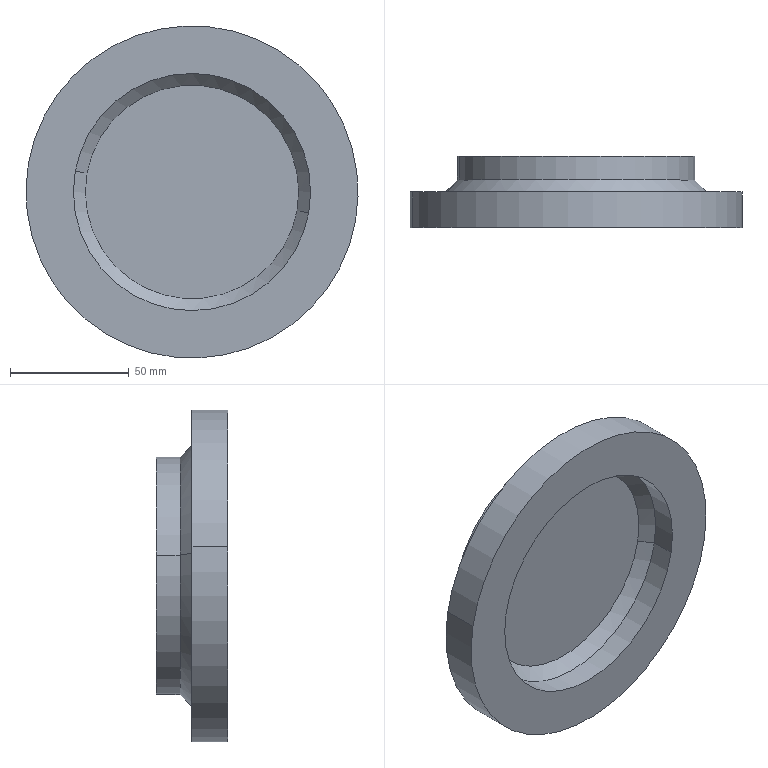Part | SolidWorks | features BaseBody 1 | 1 solid | 17 faces | box 140 x 30 x 140 mm | volume 231551 mm3 | cone 6 | cylinder 6 | plane 5 | commonest cylinder face diameters 100 x4 140 x2
STEP:
#1=CARTESIAN_POINT('',(224.832,513.635,261.862));
#2=VERTEX_POINT('',#1);
#3=CARTESIAN_POINT('',(214.987,523.635,263.616));
#4=VERTEX_POINT('',#3);
#5=CARTESIAN_POINT('',(224.832,513.635,261.862));
#6=DIRECTION('',(-0.6961,0.7071,0.1241));
#7=VECTOR('',#6,1000.);
#8=LINE('',#5,#7);
#9=EDGE_CURVE('',#2,#4,#8,.T.);
#10=ORIENTED_EDGE('',*,*,#9,.F.);
#11=CARTESIAN_POINT('',(244.522,513.635,258.352));
#12=VERTEX_POINT('',#11);
#13=CARTESIAN_POINT('',(234.677,513.635,260.107));
#14=DIRECTION('',(0.,1.,0.));
#15=DIRECTION('',(0.9845,0.,-0.1755));
#16=AXIS2_PLACEMENT_3D('',#13,#14,#15);
#17=CIRCLE('',#16,10.);
#18=EDGE_CURVE('',#12,#2,#17,.T.);
#19=ORIENTED_EDGE('',*,*,#18,.F.);
#20=CARTESIAN_POINT('',(254.367,523.635,256.597));
#21=VERTEX_POINT('',#20);
#22=CARTESIAN_POINT('',(244.522,513.635,258.352));
#23=DIRECTION('',(0.6961,0.7071,-0.1241));
#24=VECTOR('',#23,1000.);
#25=LINE('',#22,#24);
#26=EDGE_CURVE('',#12,#21,#25,.T.);
#27=ORIENTED_EDGE('',*,*,#26,.T.);
#28=CARTESIAN_POINT('',(234.677,523.635,260.107));
#29=DIRECTION('',(0.,-1.,0.));
#30=DIRECTION('',(0.9845,0.,-0.1755));
#31=AXIS2_PLACEMENT_3D('',#28,#29,#30);
#32=CIRCLE('',#31,20.);
#33=EDGE_CURVE('',#4,#21,#32,.T.);
#34=ORIENTED_EDGE('',*,*,#33,.F.);
#35=EDGE_LOOP('',(#10,#19,#27,#34));
#36=FACE_OUTER_BOUND('',#35,.T.);
#37=CARTESIAN_POINT('',(234.677,513.635,260.107));
#38=DIRECTION('',(0.,1.,0.));
#39=DIRECTION('',(-0.9845,0.,0.1755));
#40=AXIS2_PLACEMENT_3D('',#37,#38,#39);
#41=CONICAL_SURFACE('',#40,10.,0.7854);
#42=ADVANCED_FACE('',(#36),#41,.F.);
#43=ORIENTED_EDGE('',*,*,#18,.T.);
#44=CARTESIAN_POINT('',(234.677,513.635,260.107));
#45=DIRECTION('',(0.,1.,0.));
#46=DIRECTION('',(0.9845,0.,-0.1755));
#47=AXIS2_PLACEMENT_3D('',#44,#45,#46);
#48=CIRCLE('',#47,10.);
#49=EDGE_CURVE('',#2,#12,#48,.T.);
#50=ORIENTED_EDGE('',*,*,#49,.T.);
#51=EDGE_LOOP('',(#43,#50));
#52=FACE_OUTER_BOUND('',#51,.T.);
#53=CARTESIAN_POINT('',(234.677,513.635,260.107));
#54=DIRECTION('',(0.,1.,0.));
#55=DIRECTION('',(1.,0.,0.));
#56=AXIS2_PLACEMENT_3D('',#53,#54,#55);
#57=PLANE('',#56);
#58=ADVANCED_FACE('',(#52),#57,.T.);
#59=CARTESIAN_POINT('',(283.901,523.635,251.332));
#60=VERTEX_POINT('',#59);
#61=CARTESIAN_POINT('',(283.901,513.635,251.332));
#62=VERTEX_POINT('',#61);
#63=CARTESIAN_POINT('',(283.901,523.635,251.332));
#64=DIRECTION('',(0.,-1.,0.));
#65=VECTOR('',#64,1000.);
#66=LINE('',#63,#65);
#67=EDGE_CURVE('',#60,#62,#66,.T.);
#68=ORIENTED_EDGE('',*,*,#67,.F.);
#69=CARTESIAN_POINT('',(185.453,523.635,268.881));
#70=VERTEX_POINT('',#69);
#71=CARTESIAN_POINT('',(234.677,523.635,260.107));
#72=DIRECTION('',(0.,1.,0.));
#73=DIRECTION('',(0.9845,0.,-0.1755));
#74=AXIS2_PLACEMENT_3D('',#71,#72,#73);
#75=CIRCLE('',#74,50.);
#76=EDGE_CURVE('',#70,#60,#75,.T.);
#77=ORIENTED_EDGE('',*,*,#76,.F.);
#78=CARTESIAN_POINT('',(185.453,513.635,268.881));
#79=VERTEX_POINT('',#78);
#80=CARTESIAN_POINT('',(185.453,523.635,268.881));
#81=DIRECTION('',(0.,-1.,0.));
#82=VECTOR('',#81,1000.);
#83=LINE('',#80,#82);
#84=EDGE_CURVE('',#70,#79,#83,.T.);
#85=ORIENTED_EDGE('',*,*,#84,.T.);
#86=CARTESIAN_POINT('',(234.677,513.635,260.107));
#87=DIRECTION('',(0.,-1.,0.));
#88=DIRECTION('',(-0.9845,0.,0.1755));
#89=AXIS2_PLACEMENT_3D('',#86,#87,#88);
#90=CIRCLE('',#89,50.);
#91=EDGE_CURVE('',#62,#79,#90,.T.);
#92=ORIENTED_EDGE('',*,*,#91,.F.);
#93=EDGE_LOOP('',(#68,#77,#85,#92));
#94=FACE_OUTER_BOUND('',#93,.T.);
#95=CARTESIAN_POINT('',(234.677,523.635,260.107));
#96=DIRECTION('',(0.,-1.,0.));
#97=DIRECTION('',(0.9845,0.,-0.1755));
#98=AXIS2_PLACEMENT_3D('',#95,#96,#97);
#99=CYLINDRICAL_SURFACE('',#98,50.);
#100=ADVANCED_FACE('',(#94),#99,.T.);
#101=CARTESIAN_POINT('',(234.677,523.635,260.107));
#102=DIRECTION('',(0.,-1.,0.));
#103=DIRECTION('',(0.9845,0.,-0.1755));
#104=AXIS2_PLACEMENT_3D('',#101,#102,#103);
#105=CIRCLE('',#104,20.);
#106=EDGE_CURVE('',#21,#4,#105,.T.);
#107=ORIENTED_EDGE('',*,*,#106,.T.);
#108=ORIENTED_EDGE('',*,*,#33,.T.);
#109=EDGE_LOOP('',(#107,#108));
#110=FACE_BOUND('',#109,.T.);
#111=ORIENTED_EDGE('',*,*,#76,.T.);
#112=CARTESIAN_POINT('',(234.677,523.635,260.107));
#113=DIRECTION('',(0.,1.,0.));
#114=DIRECTION('',(0.9845,0.,-0.1755));
#115=AXIS2_PLACEMENT_3D('',#112,#113,#114);
#116=CIRCLE('',#115,50.);
#117=EDGE_CURVE('',#60,#70,#116,.T.);
#118=ORIENTED_EDGE('',*,*,#117,.T.);
#119=EDGE_LOOP('',(#111,#118));
#120=FACE_OUTER_BOUND('',#119,.T.);
#121=CARTESIAN_POINT('',(234.677,523.635,260.107));
#122=DIRECTION('',(0.,1.,0.));
#123=DIRECTION('',(1.,0.,0.));
#124=AXIS2_PLACEMENT_3D('',#121,#122,#123);
#125=PLANE('',#124);
#126=ADVANCED_FACE('',(#110,#120),#125,.T.);
#127=CARTESIAN_POINT('',(288.965,508.635,250.43));
#128=VERTEX_POINT('',#127);
#129=CARTESIAN_POINT('',(288.965,508.635,250.43));
#130=DIRECTION('',(0.7059,-0.697,-0.1258));
#131=VECTOR('',#130,1000.);
#132=LINE('',#129,#131);
#133=EDGE_CURVE('',#62,#128,#132,.T.);
#134=ORIENTED_EDGE('',*,*,#133,.F.);
#135=ORIENTED_EDGE('',*,*,#91,.T.);
#136=CARTESIAN_POINT('',(180.389,508.635,269.784));
#137=VERTEX_POINT('',#136);
#138=CARTESIAN_POINT('',(180.389,508.635,269.784));
#139=DIRECTION('',(-0.7059,-0.697,0.1258));
#140=VECTOR('',#139,1000.);
#141=LINE('',#138,#140);
#142=EDGE_CURVE('',#79,#137,#141,.T.);
#143=ORIENTED_EDGE('',*,*,#142,.T.);
#144=CARTESIAN_POINT('',(234.677,508.635,260.107));
#145=DIRECTION('',(0.,1.,0.));
#146=DIRECTION('',(0.9845,0.,-0.1755));
#147=AXIS2_PLACEMENT_3D('',#144,#145,#146);
#148=CIRCLE('',#147,55.144);
#149=EDGE_CURVE('',#137,#128,#148,.T.);
#150=ORIENTED_EDGE('',*,*,#149,.T.);
#151=EDGE_LOOP('',(#134,#135,#143,#150));
#152=FACE_OUTER_BOUND('',#151,.T.);
#153=CARTESIAN_POINT('',(234.677,508.635,260.107));
#154=DIRECTION('',(0.,-1.,0.));
#155=DIRECTION('',(0.9845,0.,-0.1755));
#156=AXIS2_PLACEMENT_3D('',#153,#154,#155);
#157=CONICAL_SURFACE('',#156,55.144,0.7996);
#158=ADVANCED_FACE('',(#152),#157,.T.);
#159=CARTESIAN_POINT('',(190.375,508.635,268.004));
#160=VERTEX_POINT('',#159);
#161=CARTESIAN_POINT('',(278.979,508.635,252.21));
#162=VERTEX_POINT('',#161);
#163=CARTESIAN_POINT('',(234.677,508.635,260.107));
#164=DIRECTION('',(0.,1.,0.));
#165=DIRECTION('',(0.9845,0.,-0.1755));
#166=AXIS2_PLACEMENT_3D('',#163,#164,#165);
#167=CIRCLE('',#166,45.);
#168=EDGE_CURVE('',#160,#162,#167,.T.);
#169=ORIENTED_EDGE('',*,*,#168,.F.);
#170=CARTESIAN_POINT('',(234.677,508.635,260.107));
#171=DIRECTION('',(0.,1.,0.));
#172=DIRECTION('',(0.9845,0.,-0.1755));
#173=AXIS2_PLACEMENT_3D('',#170,#171,#172);
#174=CIRCLE('',#173,45.);
#175=EDGE_CURVE('',#162,#160,#174,.T.);
#176=ORIENTED_EDGE('',*,*,#175,.F.);
#177=EDGE_LOOP('',(#169,#176));
#178=FACE_OUTER_BOUND('',#177,.T.);
#179=CARTESIAN_POINT('',(234.677,508.635,260.107));
#180=DIRECTION('',(0.,1.,0.));
#181=DIRECTION('',(1.,0.,0.));
#182=AXIS2_PLACEMENT_3D('',#179,#180,#181);
#183=PLANE('',#182);
#184=ADVANCED_FACE('',(#178),#183,.F.);
#185=CARTESIAN_POINT('',(283.901,503.635,251.332));
#186=VERTEX_POINT('',#185);
#187=CARTESIAN_POINT('',(283.901,503.635,251.332));
#188=DIRECTION('',(0.6961,-0.7071,-0.1241));
#189=VECTOR('',#188,1000.);
#190=LINE('',#187,#189);
#191=EDGE_CURVE('',#162,#186,#190,.T.);
#192=ORIENTED_EDGE('',*,*,#191,.F.);
#193=ORIENTED_EDGE('',*,*,#175,.T.);
#194=CARTESIAN_POINT('',(185.453,503.635,268.881));
#195=VERTEX_POINT('',#194);
#196=CARTESIAN_POINT('',(185.453,503.635,268.881));
#197=DIRECTION('',(-0.6961,-0.7071,0.1241));
#198=VECTOR('',#197,1000.);
#199=LINE('',#196,#198);
#200=EDGE_CURVE('',#160,#195,#199,.T.);
#201=ORIENTED_EDGE('',*,*,#200,.T.);
#202=CARTESIAN_POINT('',(234.677,503.635,260.107));
#203=DIRECTION('',(0.,-1.,0.));
#204=DIRECTION('',(-0.9845,0.,0.1755));
#205=AXIS2_PLACEMENT_3D('',#202,#203,#204);
#206=CIRCLE('',#205,50.);
#207=EDGE_CURVE('',#195,#186,#206,.T.);
#208=ORIENTED_EDGE('',*,*,#207,.T.);
#209=EDGE_LOOP('',(#192,#193,#201,#208));
#210=FACE_OUTER_BOUND('',#209,.T.);
#211=CARTESIAN_POINT('',(234.677,503.635,260.107));
#212=DIRECTION('',(0.,-1.,0.));
#213=DIRECTION('',(0.9845,0.,-0.1755));
#214=AXIS2_PLACEMENT_3D('',#211,#212,#213);
#215=CONICAL_SURFACE('',#214,50.,0.7854);
#216=ADVANCED_FACE('',(#210),#215,.F.);
#217=CARTESIAN_POINT('',(283.901,493.635,251.332));
#218=VERTEX_POINT('',#217);
#219=CARTESIAN_POINT('',(283.901,508.635,251.332));
#220=DIRECTION('',(0.,-1.,0.));
#221=VECTOR('',#220,1000.);
#222=LINE('',#219,#221);
#223=EDGE_CURVE('',#186,#218,#222,.T.);
#224=ORIENTED_EDGE('',*,*,#223,.F.);
#225=ORIENTED_EDGE('',*,*,#207,.F.);
#226=CARTESIAN_POINT('',(185.453,493.635,268.881));
#227=VERTEX_POINT('',#226);
#228=CARTESIAN_POINT('',(185.453,508.635,268.881));
#229=DIRECTION('',(0.,-1.,0.));
#230=VECTOR('',#229,1000.);
#231=LINE('',#228,#230);
#232=EDGE_CURVE('',#195,#227,#231,.T.);
#233=ORIENTED_EDGE('',*,*,#232,.T.);
#234=CARTESIAN_POINT('',(234.677,493.635,260.107));
#235=DIRECTION('',(0.,1.,0.));
#236=DIRECTION('',(0.9845,0.,-0.1755));
#237=AXIS2_PLACEMENT_3D('',#234,#235,#236);
#238=CIRCLE('',#237,50.);
#239=EDGE_CURVE('',#218,#227,#238,.T.);
#240=ORIENTED_EDGE('',*,*,#239,.F.);
#241=EDGE_LOOP('',(#224,#225,#233,#240));
#242=FACE_OUTER_BOUND('',#241,.T.);
#243=CARTESIAN_POINT('',(234.677,508.635,260.107));
#244=DIRECTION('',(0.,-1.,0.));
#245=DIRECTION('',(0.9845,0.,-0.1755));
#246=AXIS2_PLACEMENT_3D('',#243,#244,#245);
#247=CYLINDRICAL_SURFACE('',#246,50.);
#248=ADVANCED_FACE('',(#242),#247,.F.);
#249=CARTESIAN_POINT('',(303.591,508.635,247.823));
#250=VERTEX_POINT('',#249);
#251=CARTESIAN_POINT('',(303.591,493.635,247.823));
#252=VERTEX_POINT('',#251);
#253=CARTESIAN_POINT('',(303.591,508.635,247.823));
#254=DIRECTION('',(0.,-1.,0.));
#255=VECTOR('',#254,1000.);
#256=LINE('',#253,#255);
#257=EDGE_CURVE('',#250,#252,#256,.T.);
#258=ORIENTED_EDGE('',*,*,#257,.F.);
#259=CARTESIAN_POINT('',(165.763,508.635,272.391));
#260=VERTEX_POINT('',#259);
#261=CARTESIAN_POINT('',(234.677,508.635,260.107));
#262=DIRECTION('',(0.,1.,0.));
#263=DIRECTION('',(0.9845,0.,-0.1755));
#264=AXIS2_PLACEMENT_3D('',#261,#262,#263);
#265=CIRCLE('',#264,70.);
#266=EDGE_CURVE('',#260,#250,#265,.T.);
#267=ORIENTED_EDGE('',*,*,#266,.F.);
#268=CARTESIAN_POINT('',(165.763,493.635,272.391));
#269=VERTEX_POINT('',#268);
#270=CARTESIAN_POINT('',(165.763,508.635,272.391));
#271=DIRECTION('',(0.,-1.,0.));
#272=VECTOR('',#271,1000.);
#273=LINE('',#270,#272);
#274=EDGE_CURVE('',#260,#269,#273,.T.);
#275=ORIENTED_EDGE('',*,*,#274,.T.);
#276=CARTESIAN_POINT('',(234.677,493.635,260.107));
#277=DIRECTION('',(0.,1.,0.));
#278=DIRECTION('',(0.9845,0.,-0.1755));
#279=AXIS2_PLACEMENT_3D('',#276,#277,#278);
#280=CIRCLE('',#279,70.);
#281=EDGE_CURVE('',#269,#252,#280,.T.);
#282=ORIENTED_EDGE('',*,*,#281,.T.);
#283=EDGE_LOOP('',(#258,#267,#275,#282));
#284=FACE_OUTER_BOUND('',#283,.T.);
#285=CARTESIAN_POINT('',(234.677,508.635,260.107));
#286=DIRECTION('',(0.,-1.,0.));
#287=DIRECTION('',(0.9845,0.,-0.1755));
#288=AXIS2_PLACEMENT_3D('',#285,#286,#287);
#289=CYLINDRICAL_SURFACE('',#288,70.);
#290=ADVANCED_FACE('',(#284),#289,.T.);
#291=CARTESIAN_POINT('',(234.677,493.635,260.107));
#292=DIRECTION('',(0.,1.,0.));
#293=DIRECTION('',(0.9845,0.,-0.1755));
#294=AXIS2_PLACEMENT_3D('',#291,#292,#293);
#295=CIRCLE('',#294,50.);
#296=EDGE_CURVE('',#227,#218,#295,.T.);
#297=ORIENTED_EDGE('',*,*,#296,.T.);
#298=ORIENTED_EDGE('',*,*,#239,.T.);
#299=EDGE_LOOP('',(#297,#298));
#300=FACE_BOUND('',#299,.T.);
#301=ORIENTED_EDGE('',*,*,#281,.F.);
#302=CARTESIAN_POINT('',(234.677,493.635,260.107));
#303=DIRECTION('',(0.,1.,0.));
#304=DIRECTION('',(0.9845,0.,-0.1755));
#305=AXIS2_PLACEMENT_3D('',#302,#303,#304);
#306=CIRCLE('',#305,70.);
#307=EDGE_CURVE('',#252,#269,#306,.T.);
#308=ORIENTED_EDGE('',*,*,#307,.F.);
#309=EDGE_LOOP('',(#301,#308));
#310=FACE_OUTER_BOUND('',#309,.T.);
#311=CARTESIAN_POINT('',(234.677,493.635,260.107));
#312=DIRECTION('',(0.,1.,0.));
#313=DIRECTION('',(1.,0.,0.));
#314=AXIS2_PLACEMENT_3D('',#311,#312,#313);
#315=PLANE('',#314);
#316=ADVANCED_FACE('',(#300,#310),#315,.F.);
#317=ORIENTED_EDGE('',*,*,#149,.F.);
#318=CARTESIAN_POINT('',(234.677,508.635,260.107));
#319=DIRECTION('',(0.,1.,0.));
#320=DIRECTION('',(0.9845,0.,-0.1755));
#321=AXIS2_PLACEMENT_3D('',#318,#319,#320);
#322=CIRCLE('',#321,55.144);
#323=EDGE_CURVE('',#128,#137,#322,.T.);
#324=ORIENTED_EDGE('',*,*,#323,.F.);
#325=EDGE_LOOP('',(#317,#324));
#326=FACE_BOUND('',#325,.T.);
#327=ORIENTED_EDGE('',*,*,#266,.T.);
#328=CARTESIAN_POINT('',(234.677,508.635,260.107));
#329=DIRECTION('',(0.,1.,0.));
#330=DIRECTION('',(0.9845,0.,-0.1755));
#331=AXIS2_PLACEMENT_3D('',#328,#329,#330);
#332=CIRCLE('',#331,70.);
#333=EDGE_CURVE('',#250,#260,#332,.T.);
#334=ORIENTED_EDGE('',*,*,#333,.T.);
#335=EDGE_LOOP('',(#327,#334));
#336=FACE_OUTER_BOUND('',#335,.T.);
#337=CARTESIAN_POINT('',(234.677,508.635,260.107));
#338=DIRECTION('',(0.,1.,0.));
#339=DIRECTION('',(1.,0.,0.));
#340=AXIS2_PLACEMENT_3D('',#337,#338,#339);
#341=PLANE('',#340);
#342=ADVANCED_FACE('',(#326,#336),#341,.T.);
#343=ORIENTED_EDGE('',*,*,#333,.F.);
#344=ORIENTED_EDGE('',*,*,#257,.T.);
#345=ORIENTED_EDGE('',*,*,#307,.T.);
#346=ORIENTED_EDGE('',*,*,#274,.F.);
#347=EDGE_LOOP('',(#343,#344,#345,#346));
#348=FACE_OUTER_BOUND('',#347,.T.);
#349=CARTESIAN_POINT('',(234.677,508.635,260.107));
#350=DIRECTION('',(0.,-1.,0.));
#351=DIRECTION('',(0.9845,0.,-0.1755));
#352=AXIS2_PLACEMENT_3D('',#349,#350,#351);
#353=CYLINDRICAL_SURFACE('',#352,70.);
#354=ADVANCED_FACE('',(#348),#353,.T.);
#355=CARTESIAN_POINT('',(234.677,503.635,260.107));
#356=DIRECTION('',(0.,-1.,0.));
#357=DIRECTION('',(-0.9845,0.,0.1755));
#358=AXIS2_PLACEMENT_3D('',#355,#356,#357);
#359=CIRCLE('',#358,50.);
#360=EDGE_CURVE('',#186,#195,#359,.T.);
#361=ORIENTED_EDGE('',*,*,#360,.F.);
#362=ORIENTED_EDGE('',*,*,#223,.T.);
#363=ORIENTED_EDGE('',*,*,#296,.F.);
#364=ORIENTED_EDGE('',*,*,#232,.F.);
#365=EDGE_LOOP('',(#361,#362,#363,#364));
#366=FACE_OUTER_BOUND('',#365,.T.);
#367=CARTESIAN_POINT('',(234.677,508.635,260.107));
#368=DIRECTION('',(0.,-1.,0.));
#369=DIRECTION('',(0.9845,0.,-0.1755));
#370=AXIS2_PLACEMENT_3D('',#367,#368,#369);
#371=CYLINDRICAL_SURFACE('',#370,50.);
#372=ADVANCED_FACE('',(#366),#371,.F.);
#373=ORIENTED_EDGE('',*,*,#168,.T.);
#374=ORIENTED_EDGE('',*,*,#191,.T.);
#375=ORIENTED_EDGE('',*,*,#360,.T.);
#376=ORIENTED_EDGE('',*,*,#200,.F.);
#377=EDGE_LOOP('',(#373,#374,#375,#376));
#378=FACE_OUTER_BOUND('',#377,.T.);
#379=CARTESIAN_POINT('',(234.677,503.635,260.107));
#380=DIRECTION('',(0.,-1.,0.));
#381=DIRECTION('',(0.9845,0.,-0.1755));
#382=AXIS2_PLACEMENT_3D('',#379,#380,#381);
#383=CONICAL_SURFACE('',#382,50.,0.7854);
#384=ADVANCED_FACE('',(#378),#383,.F.);
#385=CARTESIAN_POINT('',(234.677,513.635,260.107));
#386=DIRECTION('',(0.,-1.,0.));
#387=DIRECTION('',(-0.9845,0.,0.1755));
#388=AXIS2_PLACEMENT_3D('',#385,#386,#387);
#389=CIRCLE('',#388,50.);
#390=EDGE_CURVE('',#79,#62,#389,.T.);
#391=ORIENTED_EDGE('',*,*,#390,.T.);
#392=ORIENTED_EDGE('',*,*,#133,.T.);
#393=ORIENTED_EDGE('',*,*,#323,.T.);
#394=ORIENTED_EDGE('',*,*,#142,.F.);
#395=EDGE_LOOP('',(#391,#392,#393,#394));
#396=FACE_OUTER_BOUND('',#395,.T.);
#397=CARTESIAN_POINT('',(234.677,508.635,260.107));
#398=DIRECTION('',(0.,-1.,0.));
#399=DIRECTION('',(0.9845,0.,-0.1755));
#400=AXIS2_PLACEMENT_3D('',#397,#398,#399);
#401=CONICAL_SURFACE('',#400,55.144,0.7996);
#402=ADVANCED_FACE('',(#396),#401,.T.);
#403=ORIENTED_EDGE('',*,*,#117,.F.);
#404=ORIENTED_EDGE('',*,*,#67,.T.);
#405=ORIENTED_EDGE('',*,*,#390,.F.);
#406=ORIENTED_EDGE('',*,*,#84,.F.);
#407=EDGE_LOOP('',(#403,#404,#405,#406));
#408=FACE_OUTER_BOUND('',#407,.T.);
#409=CARTESIAN_POINT('',(234.677,523.635,260.107));
#410=DIRECTION('',(0.,-1.,0.));
#411=DIRECTION('',(0.9845,0.,-0.1755));
#412=AXIS2_PLACEMENT_3D('',#409,#410,#411);
#413=CYLINDRICAL_SURFACE('',#412,50.);
#414=ADVANCED_FACE('',(#408),#413,.T.);
#415=ORIENTED_EDGE('',*,*,#49,.F.);
#416=ORIENTED_EDGE('',*,*,#9,.T.);
#417=ORIENTED_EDGE('',*,*,#106,.F.);
#418=ORIENTED_EDGE('',*,*,#26,.F.);
#419=EDGE_LOOP('',(#415,#416,#417,#418));
#420=FACE_OUTER_BOUND('',#419,.T.);
#421=CARTESIAN_POINT('',(234.677,513.635,260.107));
#422=DIRECTION('',(0.,1.,0.));
#423=DIRECTION('',(-0.9845,0.,0.1755));
#424=AXIS2_PLACEMENT_3D('',#421,#422,#423);
#425=CONICAL_SURFACE('',#424,10.,0.7854);
#426=ADVANCED_FACE('',(#420),#425,.F.);
#427=CLOSED_SHELL('',(#42,#58,#100,#126,#158,#184,#216,#248,#290,#316,#342,#354,#372,#384,#402,#414,#426));
#428=MANIFOLD_SOLID_BREP('',#427);
#429=CARTESIAN_POINT('',(0.,0.,0.));
#430=DIRECTION('',(0.,0.,1.));
#431=DIRECTION('',(1.,0.,0.));
#432=AXIS2_PLACEMENT_3D('',#429,#430,#431);
#433=(LENGTH_UNIT()NAMED_UNIT(*)SI_UNIT(.MILLI.,.METRE.));
#434=UNCERTAINTY_MEASURE_WITH_UNIT(LENGTH_MEASURE(0.00001),#433,'','');
#435=(NAMED_UNIT(*)PLANE_ANGLE_UNIT()SI_UNIT($,.RADIAN.));
#436=(NAMED_UNIT(*)SI_UNIT($,.STERADIAN.)SOLID_ANGLE_UNIT());
#437=(GEOMETRIC_REPRESENTATION_CONTEXT(3)GLOBAL_UNCERTAINTY_ASSIGNED_CONTEXT((#434))GLOBAL_UNIT_ASSIGNED_CONTEXT((#433,#435,#436))REPRESENTATION_CONTEXT('',''));
#438=ADVANCED_BREP_SHAPE_REPRESENTATION('',(#428,#432),#437);